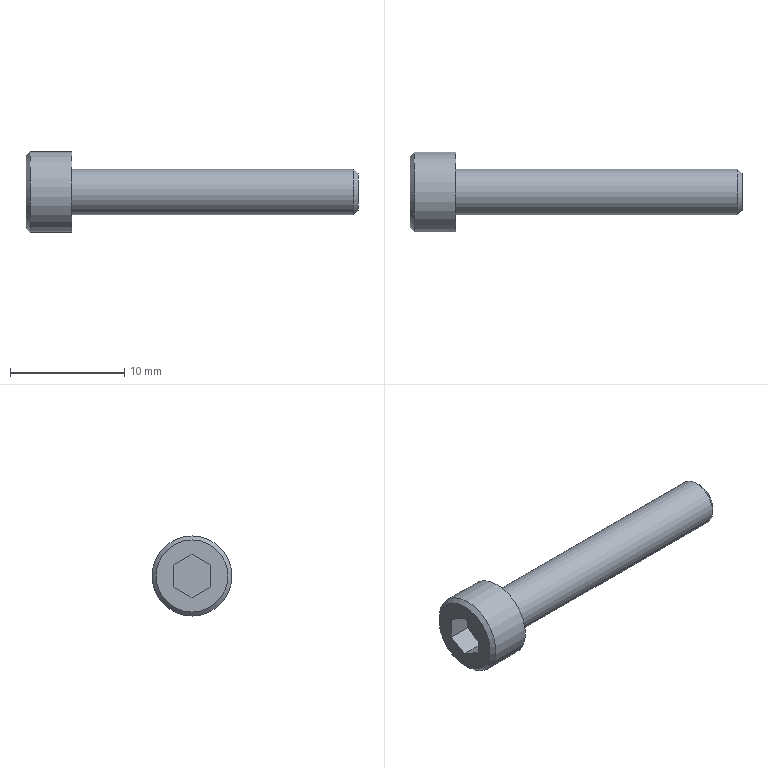Part | STEP file | M4.00-25.00 | 1 solid | 14 faces | box 29 x 7 x 7 mm | volume 447.208 mm3 | plane 10 | cylinder 2 | cone 2 | commonest cylinder face diameters 4 x1 7 x1